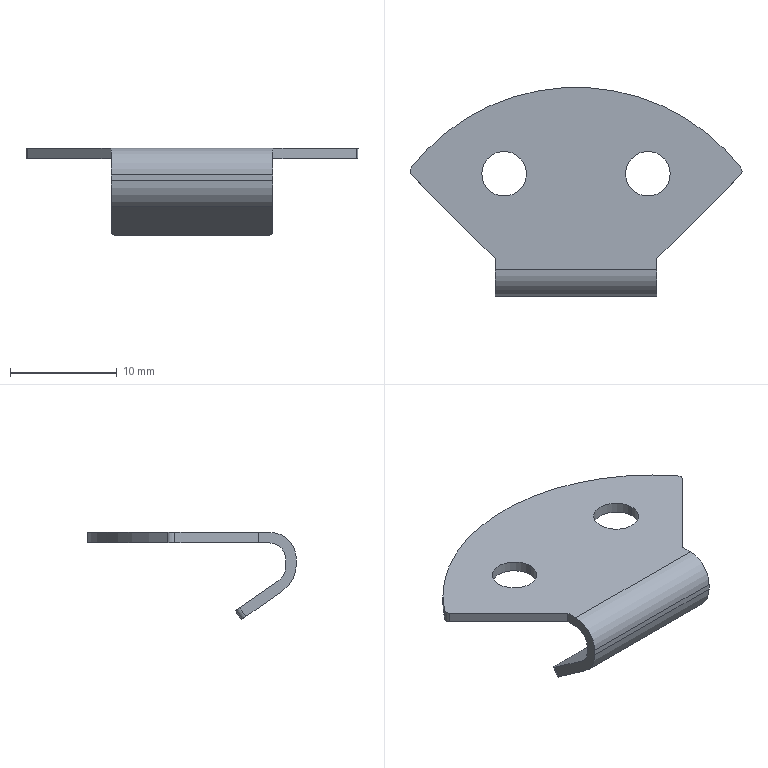Part | SolidWorks | features BaseBody 1 | 1 solid | 24 faces | box 31.176 x 19.62 x 8.2 mm | volume 515.875 mm3 | cylinder 13 | plane 11 | commonest cylinder face diameters 1 x4 4.2 x4 3 x2 5 x1 6 x1 39.24 x1
STEP:
#1=CARTESIAN_POINT('',(8.85,0.,0.));
#2=VERTEX_POINT('',#1);
#3=CARTESIAN_POINT('',(4.65,0.,0.));
#4=VERTEX_POINT('',#3);
#5=CARTESIAN_POINT('',(6.75,0.,0.));
#6=DIRECTION('',(0.,0.,-1.));
#7=DIRECTION('',(-1.,0.,0.));
#8=AXIS2_PLACEMENT_3D('',#5,#6,#7);
#9=CIRCLE('',#8,2.1);
#10=EDGE_CURVE('',#2,#4,#9,.T.);
#11=ORIENTED_EDGE('',*,*,#10,.T.);
#12=CARTESIAN_POINT('',(4.65,0.,1.));
#13=VERTEX_POINT('',#12);
#14=CARTESIAN_POINT('',(4.65,0.,0.));
#15=DIRECTION('',(0.,0.,1.));
#16=VECTOR('',#15,1000.);
#17=LINE('',#14,#16);
#18=EDGE_CURVE('',#4,#13,#17,.T.);
#19=ORIENTED_EDGE('',*,*,#18,.T.);
#20=CARTESIAN_POINT('',(8.85,0.,1.));
#21=VERTEX_POINT('',#20);
#22=CARTESIAN_POINT('',(6.75,0.,1.));
#23=DIRECTION('',(0.,0.,-1.));
#24=DIRECTION('',(1.,0.,0.));
#25=AXIS2_PLACEMENT_3D('',#22,#23,#24);
#26=CIRCLE('',#25,2.1);
#27=EDGE_CURVE('',#21,#13,#26,.T.);
#28=ORIENTED_EDGE('',*,*,#27,.F.);
#29=CARTESIAN_POINT('',(8.85,0.,0.));
#30=DIRECTION('',(0.,0.,1.));
#31=VECTOR('',#30,1000.);
#32=LINE('',#29,#31);
#33=EDGE_CURVE('',#2,#21,#32,.T.);
#34=ORIENTED_EDGE('',*,*,#33,.F.);
#35=EDGE_LOOP('',(#11,#19,#28,#34));
#36=FACE_OUTER_BOUND('',#35,.T.);
#37=CARTESIAN_POINT('',(6.75,0.,0.));
#38=DIRECTION('',(0.,0.,1.));
#39=DIRECTION('',(1.,0.,0.));
#40=AXIS2_PLACEMENT_3D('',#37,#38,#39);
#41=CYLINDRICAL_SURFACE('',#40,2.1);
#42=ADVANCED_FACE('',(#36),#41,.F.);
#43=CARTESIAN_POINT('',(-4.65,0.,0.));
#44=VERTEX_POINT('',#43);
#45=CARTESIAN_POINT('',(-8.85,0.,0.));
#46=VERTEX_POINT('',#45);
#47=CARTESIAN_POINT('',(-6.75,0.,0.));
#48=DIRECTION('',(0.,0.,-1.));
#49=DIRECTION('',(-1.,0.,0.));
#50=AXIS2_PLACEMENT_3D('',#47,#48,#49);
#51=CIRCLE('',#50,2.1);
#52=EDGE_CURVE('',#44,#46,#51,.T.);
#53=ORIENTED_EDGE('',*,*,#52,.T.);
#54=CARTESIAN_POINT('',(-8.85,0.,1.));
#55=VERTEX_POINT('',#54);
#56=CARTESIAN_POINT('',(-8.85,0.,0.));
#57=DIRECTION('',(0.,0.,1.));
#58=VECTOR('',#57,1000.);
#59=LINE('',#56,#58);
#60=EDGE_CURVE('',#46,#55,#59,.T.);
#61=ORIENTED_EDGE('',*,*,#60,.T.);
#62=CARTESIAN_POINT('',(-4.65,0.,1.));
#63=VERTEX_POINT('',#62);
#64=CARTESIAN_POINT('',(-6.75,0.,1.));
#65=DIRECTION('',(0.,0.,-1.));
#66=DIRECTION('',(-1.,0.,0.));
#67=AXIS2_PLACEMENT_3D('',#64,#65,#66);
#68=CIRCLE('',#67,2.1);
#69=EDGE_CURVE('',#63,#55,#68,.T.);
#70=ORIENTED_EDGE('',*,*,#69,.F.);
#71=CARTESIAN_POINT('',(-4.65,0.,0.));
#72=DIRECTION('',(0.,0.,1.));
#73=VECTOR('',#72,1000.);
#74=LINE('',#71,#73);
#75=EDGE_CURVE('',#44,#63,#74,.T.);
#76=ORIENTED_EDGE('',*,*,#75,.F.);
#77=EDGE_LOOP('',(#53,#61,#70,#76));
#78=FACE_OUTER_BOUND('',#77,.T.);
#79=CARTESIAN_POINT('',(-6.75,0.,0.));
#80=DIRECTION('',(0.,0.,1.));
#81=DIRECTION('',(1.,0.,0.));
#82=AXIS2_PLACEMENT_3D('',#79,#80,#81);
#83=CYLINDRICAL_SURFACE('',#82,2.1);
#84=ADVANCED_FACE('',(#78),#83,.F.);
#85=CARTESIAN_POINT('',(-15.441,-0.1087,0.));
#86=VERTEX_POINT('',#85);
#87=CARTESIAN_POINT('',(-7.6,-7.95,0.));
#88=VERTEX_POINT('',#87);
#89=CARTESIAN_POINT('',(-15.441,-0.1087,0.));
#90=DIRECTION('',(0.7071,-0.7071,0.));
#91=VECTOR('',#90,1000.);
#92=LINE('',#89,#91);
#93=EDGE_CURVE('',#86,#88,#92,.T.);
#94=ORIENTED_EDGE('',*,*,#93,.T.);
#95=CARTESIAN_POINT('',(-7.6,-7.95,1.));
#96=VERTEX_POINT('',#95);
#97=CARTESIAN_POINT('',(-7.6,-7.95,0.));
#98=DIRECTION('',(0.,0.,1.));
#99=VECTOR('',#98,1000.);
#100=LINE('',#97,#99);
#101=EDGE_CURVE('',#88,#96,#100,.T.);
#102=ORIENTED_EDGE('',*,*,#101,.T.);
#103=CARTESIAN_POINT('',(-15.441,-0.1087,1.));
#104=VERTEX_POINT('',#103);
#105=CARTESIAN_POINT('',(-15.441,-0.1087,1.));
#106=DIRECTION('',(0.7071,-0.7071,0.));
#107=VECTOR('',#106,1000.);
#108=LINE('',#105,#107);
#109=EDGE_CURVE('',#104,#96,#108,.T.);
#110=ORIENTED_EDGE('',*,*,#109,.F.);
#111=CARTESIAN_POINT('',(-15.441,-0.1087,1.));
#112=DIRECTION('',(0.,0.,-1.));
#113=VECTOR('',#112,1000.);
#114=LINE('',#111,#113);
#115=EDGE_CURVE('',#104,#86,#114,.T.);
#116=ORIENTED_EDGE('',*,*,#115,.T.);
#117=EDGE_LOOP('',(#94,#102,#110,#116));
#118=FACE_OUTER_BOUND('',#117,.T.);
#119=CARTESIAN_POINT('',(-15.75,0.2,0.));
#120=DIRECTION('',(-0.7071,-0.7071,0.));
#121=DIRECTION('',(-0.7071,0.7071,0.));
#122=AXIS2_PLACEMENT_3D('',#119,#120,#121);
#123=PLANE('',#122);
#124=ADVANCED_FACE('',(#118),#123,.T.);
#125=CARTESIAN_POINT('',(-7.6,-9.,1.));
#126=VERTEX_POINT('',#125);
#127=CARTESIAN_POINT('',(7.6,-9.,1.));
#128=VERTEX_POINT('',#127);
#129=CARTESIAN_POINT('',(-7.6,-9.,1.));
#130=DIRECTION('',(1.,0.,0.));
#131=VECTOR('',#130,1000.);
#132=LINE('',#129,#131);
#133=EDGE_CURVE('',#126,#128,#132,.T.);
#134=ORIENTED_EDGE('',*,*,#133,.F.);
#135=CARTESIAN_POINT('',(-7.6,-11.5,-1.5));
#136=VERTEX_POINT('',#135);
#137=CARTESIAN_POINT('',(-7.6,-9.,-1.5));
#138=DIRECTION('',(-1.,0.,0.));
#139=DIRECTION('',(0.,-1.,0.));
#140=AXIS2_PLACEMENT_3D('',#137,#138,#139);
#141=CIRCLE('',#140,2.5);
#142=EDGE_CURVE('',#136,#126,#141,.T.);
#143=ORIENTED_EDGE('',*,*,#142,.F.);
#144=CARTESIAN_POINT('',(7.6,-11.5,-1.5));
#145=VERTEX_POINT('',#144);
#146=CARTESIAN_POINT('',(-7.6,-11.5,-1.5));
#147=DIRECTION('',(1.,0.,0.));
#148=VECTOR('',#147,1000.);
#149=LINE('',#146,#148);
#150=EDGE_CURVE('',#136,#145,#149,.T.);
#151=ORIENTED_EDGE('',*,*,#150,.T.);
#152=CARTESIAN_POINT('',(7.6,-9.,-1.5));
#153=DIRECTION('',(1.,0.,0.));
#154=DIRECTION('',(0.,0.,1.));
#155=AXIS2_PLACEMENT_3D('',#152,#153,#154);
#156=CIRCLE('',#155,2.5);
#157=EDGE_CURVE('',#128,#145,#156,.T.);
#158=ORIENTED_EDGE('',*,*,#157,.F.);
#159=EDGE_LOOP('',(#134,#143,#151,#158));
#160=FACE_OUTER_BOUND('',#159,.T.);
#161=CARTESIAN_POINT('',(-56.813,-9.,-1.5));
#162=DIRECTION('',(1.,0.,0.));
#163=DIRECTION('',(0.,0.,1.));
#164=AXIS2_PLACEMENT_3D('',#161,#162,#163);
#165=CYLINDRICAL_SURFACE('',#164,2.5);
#166=ADVANCED_FACE('',(#160),#165,.T.);
#167=CARTESIAN_POINT('',(7.6,-11.5,-2.037));
#168=VERTEX_POINT('',#167);
#169=CARTESIAN_POINT('',(7.6,-11.5,-1.5));
#170=DIRECTION('',(0.,0.,-1.));
#171=VECTOR('',#170,1000.);
#172=LINE('',#169,#171);
#173=EDGE_CURVE('',#145,#168,#172,.T.);
#174=ORIENTED_EDGE('',*,*,#173,.F.);
#175=ORIENTED_EDGE('',*,*,#150,.F.);
#176=CARTESIAN_POINT('',(-7.6,-11.5,-2.037));
#177=VERTEX_POINT('',#176);
#178=CARTESIAN_POINT('',(-7.6,-11.5,-2.037));
#179=DIRECTION('',(0.,0.,1.));
#180=VECTOR('',#179,1000.);
#181=LINE('',#178,#180);
#182=EDGE_CURVE('',#177,#136,#181,.T.);
#183=ORIENTED_EDGE('',*,*,#182,.F.);
#184=CARTESIAN_POINT('',(7.6,-11.5,-2.037));
#185=DIRECTION('',(-1.,0.,0.));
#186=VECTOR('',#185,1000.);
#187=LINE('',#184,#186);
#188=EDGE_CURVE('',#168,#177,#187,.T.);
#189=ORIENTED_EDGE('',*,*,#188,.F.);
#190=EDGE_LOOP('',(#174,#175,#183,#189));
#191=FACE_OUTER_BOUND('',#190,.T.);
#192=CARTESIAN_POINT('',(-7.6,-11.5,0.));
#193=DIRECTION('',(0.,-1.,0.));
#194=DIRECTION('',(0.,0.,-1.));
#195=AXIS2_PLACEMENT_3D('',#192,#193,#194);
#196=PLANE('',#195);
#197=ADVANCED_FACE('',(#191),#196,.T.);
#198=CARTESIAN_POINT('',(7.6,-10.219,-4.496));
#199=VERTEX_POINT('',#198);
#200=CARTESIAN_POINT('',(-7.6,-10.219,-4.496));
#201=VERTEX_POINT('',#200);
#202=CARTESIAN_POINT('',(7.6,-10.219,-4.496));
#203=DIRECTION('',(-1.,0.,0.));
#204=VECTOR('',#203,1000.);
#205=LINE('',#202,#204);
#206=EDGE_CURVE('',#199,#201,#205,.T.);
#207=ORIENTED_EDGE('',*,*,#206,.F.);
#208=CARTESIAN_POINT('',(7.6,-8.5,-2.037));
#209=DIRECTION('',(1.,0.,0.));
#210=DIRECTION('',(0.,-1.,0.));
#211=AXIS2_PLACEMENT_3D('',#208,#209,#210);
#212=CIRCLE('',#211,3.);
#213=EDGE_CURVE('',#168,#199,#212,.T.);
#214=ORIENTED_EDGE('',*,*,#213,.F.);
#215=ORIENTED_EDGE('',*,*,#188,.T.);
#216=CARTESIAN_POINT('',(-7.6,-8.5,-2.037));
#217=DIRECTION('',(-1.,0.,0.));
#218=DIRECTION('',(0.,-0.5732,-0.8194));
#219=AXIS2_PLACEMENT_3D('',#216,#217,#218);
#220=CIRCLE('',#219,3.);
#221=EDGE_CURVE('',#201,#177,#220,.T.);
#222=ORIENTED_EDGE('',*,*,#221,.F.);
#223=EDGE_LOOP('',(#207,#214,#215,#222));
#224=FACE_OUTER_BOUND('',#223,.T.);
#225=CARTESIAN_POINT('',(56.813,-8.5,-2.037));
#226=DIRECTION('',(-1.,0.,0.));
#227=DIRECTION('',(0.,-0.5732,-0.8194));
#228=AXIS2_PLACEMENT_3D('',#225,#226,#227);
#229=CYLINDRICAL_SURFACE('',#228,3.);
#230=ADVANCED_FACE('',(#224),#229,.T.);
#231=CARTESIAN_POINT('',(-7.1,-6.353,-7.2));
#232=VERTEX_POINT('',#231);
#233=CARTESIAN_POINT('',(7.1,-6.353,-7.2));
#234=VERTEX_POINT('',#233);
#235=CARTESIAN_POINT('',(-7.1,-6.353,-7.2));
#236=DIRECTION('',(1.,0.,0.));
#237=VECTOR('',#236,1000.);
#238=LINE('',#235,#237);
#239=EDGE_CURVE('',#232,#234,#238,.T.);
#240=ORIENTED_EDGE('',*,*,#239,.F.);
#241=CARTESIAN_POINT('',(-7.1,-5.78,-6.381));
#242=VERTEX_POINT('',#241);
#243=CARTESIAN_POINT('',(-7.1,-5.78,-6.381));
#244=DIRECTION('',(0.,-0.5732,-0.8194));
#245=VECTOR('',#244,1000.);
#246=LINE('',#243,#245);
#247=EDGE_CURVE('',#242,#232,#246,.T.);
#248=ORIENTED_EDGE('',*,*,#247,.F.);
#249=CARTESIAN_POINT('',(7.1,-5.78,-6.381));
#250=VERTEX_POINT('',#249);
#251=CARTESIAN_POINT('',(-7.1,-5.78,-6.381));
#252=DIRECTION('',(1.,0.,0.));
#253=VECTOR('',#252,1000.);
#254=LINE('',#251,#253);
#255=EDGE_CURVE('',#242,#250,#254,.T.);
#256=ORIENTED_EDGE('',*,*,#255,.T.);
#257=CARTESIAN_POINT('',(7.1,-6.353,-7.2));
#258=DIRECTION('',(0.,0.5732,0.8194));
#259=VECTOR('',#258,1000.);
#260=LINE('',#257,#259);
#261=EDGE_CURVE('',#234,#250,#260,.T.);
#262=ORIENTED_EDGE('',*,*,#261,.F.);
#263=EDGE_LOOP('',(#240,#248,#256,#262));
#264=FACE_OUTER_BOUND('',#263,.T.);
#265=CARTESIAN_POINT('',(-7.6,-6.353,-7.2));
#266=DIRECTION('',(0.,0.8194,-0.5732));
#267=DIRECTION('',(-1.,0.,0.));
#268=AXIS2_PLACEMENT_3D('',#265,#266,#267);
#269=PLANE('',#268);
#270=ADVANCED_FACE('',(#264),#269,.T.);
#271=CARTESIAN_POINT('',(7.6,-6.763,-6.913));
#272=VERTEX_POINT('',#271);
#273=CARTESIAN_POINT('',(7.6,-10.219,-4.496));
#274=DIRECTION('',(0.,0.8194,-0.5732));
#275=VECTOR('',#274,1000.);
#276=LINE('',#273,#275);
#277=EDGE_CURVE('',#199,#272,#276,.T.);
#278=ORIENTED_EDGE('',*,*,#277,.F.);
#279=ORIENTED_EDGE('',*,*,#206,.T.);
#280=CARTESIAN_POINT('',(-7.6,-6.763,-6.913));
#281=VERTEX_POINT('',#280);
#282=CARTESIAN_POINT('',(-7.6,-10.219,-4.496));
#283=DIRECTION('',(0.,0.8194,-0.5732));
#284=VECTOR('',#283,1000.);
#285=LINE('',#282,#284);
#286=EDGE_CURVE('',#201,#281,#285,.T.);
#287=ORIENTED_EDGE('',*,*,#286,.T.);
#288=CARTESIAN_POINT('',(-7.1,-6.763,-6.913));
#289=DIRECTION('',(0.,-0.5732,-0.8194));
#290=DIRECTION('',(-1.,0.,0.));
#291=AXIS2_PLACEMENT_3D('',#288,#289,#290);
#292=CIRCLE('',#291,0.5);
#293=EDGE_CURVE('',#281,#232,#292,.T.);
#294=ORIENTED_EDGE('',*,*,#293,.T.);
#295=ORIENTED_EDGE('',*,*,#239,.T.);
#296=CARTESIAN_POINT('',(7.1,-6.763,-6.913));
#297=DIRECTION('',(0.,-0.5732,-0.8194));
#298=DIRECTION('',(0.,0.8194,-0.5732));
#299=AXIS2_PLACEMENT_3D('',#296,#297,#298);
#300=CIRCLE('',#299,0.5);
#301=EDGE_CURVE('',#234,#272,#300,.T.);
#302=ORIENTED_EDGE('',*,*,#301,.T.);
#303=EDGE_LOOP('',(#278,#279,#287,#294,#295,#302));
#304=FACE_OUTER_BOUND('',#303,.T.);
#305=CARTESIAN_POINT('',(-7.6,-11.5,-3.6));
#306=DIRECTION('',(0.,-0.5732,-0.8194));
#307=DIRECTION('',(0.,-0.8194,0.5732));
#308=AXIS2_PLACEMENT_3D('',#305,#306,#307);
#309=PLANE('',#308);
#310=ADVANCED_FACE('',(#304),#309,.T.);
#311=CARTESIAN_POINT('',(-7.6,-6.19,-6.094));
#312=VERTEX_POINT('',#311);
#313=CARTESIAN_POINT('',(-7.6,-6.19,-6.094));
#314=DIRECTION('',(0.,-0.5732,-0.8194));
#315=VECTOR('',#314,1000.);
#316=LINE('',#313,#315);
#317=EDGE_CURVE('',#312,#281,#316,.T.);
#318=ORIENTED_EDGE('',*,*,#317,.F.);
#319=CARTESIAN_POINT('',(-7.1,-6.19,-6.094));
#320=DIRECTION('',(0.,0.5732,0.8194));
#321=DIRECTION('',(0.,0.8194,-0.5732));
#322=AXIS2_PLACEMENT_3D('',#319,#320,#321);
#323=CIRCLE('',#322,0.5);
#324=EDGE_CURVE('',#242,#312,#323,.T.);
#325=ORIENTED_EDGE('',*,*,#324,.F.);
#326=ORIENTED_EDGE('',*,*,#247,.T.);
#327=ORIENTED_EDGE('',*,*,#293,.F.);
#328=EDGE_LOOP('',(#318,#325,#326,#327));
#329=FACE_OUTER_BOUND('',#328,.T.);
#330=CARTESIAN_POINT('',(-7.1,6.249,11.69));
#331=DIRECTION('',(0.,-0.5732,-0.8194));
#332=DIRECTION('',(-1.,0.,0.));
#333=AXIS2_PLACEMENT_3D('',#330,#331,#332);
#334=CYLINDRICAL_SURFACE('',#333,0.5);
#335=ADVANCED_FACE('',(#329),#334,.T.);
#336=ORIENTED_EDGE('',*,*,#286,.F.);
#337=ORIENTED_EDGE('',*,*,#221,.T.);
#338=ORIENTED_EDGE('',*,*,#182,.T.);
#339=ORIENTED_EDGE('',*,*,#142,.T.);
#340=CARTESIAN_POINT('',(-7.6,-7.95,1.));
#341=DIRECTION('',(0.,-1.,0.));
#342=VECTOR('',#341,1000.);
#343=LINE('',#340,#342);
#344=EDGE_CURVE('',#96,#126,#343,.T.);
#345=ORIENTED_EDGE('',*,*,#344,.F.);
#346=ORIENTED_EDGE('',*,*,#101,.F.);
#347=CARTESIAN_POINT('',(-7.6,-9.,0.));
#348=VERTEX_POINT('',#347);
#349=CARTESIAN_POINT('',(-7.6,-7.95,0.));
#350=DIRECTION('',(0.,-1.,0.));
#351=VECTOR('',#350,1000.);
#352=LINE('',#349,#351);
#353=EDGE_CURVE('',#88,#348,#352,.T.);
#354=ORIENTED_EDGE('',*,*,#353,.T.);
#355=CARTESIAN_POINT('',(-7.6,-10.5,-1.5));
#356=VERTEX_POINT('',#355);
#357=CARTESIAN_POINT('',(-7.6,-9.,-1.5));
#358=DIRECTION('',(1.,0.,0.));
#359=DIRECTION('',(0.,0.,1.));
#360=AXIS2_PLACEMENT_3D('',#357,#358,#359);
#361=CIRCLE('',#360,1.5);
#362=EDGE_CURVE('',#348,#356,#361,.T.);
#363=ORIENTED_EDGE('',*,*,#362,.T.);
#364=CARTESIAN_POINT('',(-7.6,-10.5,-2.298));
#365=VERTEX_POINT('',#364);
#366=CARTESIAN_POINT('',(-7.6,-10.5,-2.298));
#367=DIRECTION('',(0.,0.,1.));
#368=VECTOR('',#367,1000.);
#369=LINE('',#366,#368);
#370=EDGE_CURVE('',#365,#356,#369,.T.);
#371=ORIENTED_EDGE('',*,*,#370,.F.);
#372=CARTESIAN_POINT('',(-7.6,-9.86,-3.527));
#373=VERTEX_POINT('',#372);
#374=CARTESIAN_POINT('',(-7.6,-9.,-2.298));
#375=DIRECTION('',(1.,0.,0.));
#376=DIRECTION('',(0.,-1.,0.));
#377=AXIS2_PLACEMENT_3D('',#374,#375,#376);
#378=CIRCLE('',#377,1.5);
#379=EDGE_CURVE('',#365,#373,#378,.T.);
#380=ORIENTED_EDGE('',*,*,#379,.T.);
#381=CARTESIAN_POINT('',(-7.6,-6.19,-6.094));
#382=DIRECTION('',(0.,-0.8194,0.5732));
#383=VECTOR('',#382,1000.);
#384=LINE('',#381,#383);
#385=EDGE_CURVE('',#312,#373,#384,.T.);
#386=ORIENTED_EDGE('',*,*,#385,.F.);
#387=ORIENTED_EDGE('',*,*,#317,.T.);
#388=EDGE_LOOP('',(#336,#337,#338,#339,#345,#346,#354,#363,#371,#380,#386,#387));
#389=FACE_OUTER_BOUND('',#388,.T.);
#390=CARTESIAN_POINT('',(-7.6,-7.95,0.));
#391=DIRECTION('',(-1.,0.,0.));
#392=DIRECTION('',(0.,0.,1.));
#393=AXIS2_PLACEMENT_3D('',#390,#391,#392);
#394=PLANE('',#393);
#395=ADVANCED_FACE('',(#389),#394,.T.);
#396=CARTESIAN_POINT('',(7.6,-10.5,-1.5));
#397=VERTEX_POINT('',#396);
#398=CARTESIAN_POINT('',(7.6,-9.,0.));
#399=VERTEX_POINT('',#398);
#400=CARTESIAN_POINT('',(7.6,-9.,-1.5));
#401=DIRECTION('',(-1.,0.,0.));
#402=DIRECTION('',(0.,-1.,0.));
#403=AXIS2_PLACEMENT_3D('',#400,#401,#402);
#404=CIRCLE('',#403,1.5);
#405=EDGE_CURVE('',#397,#399,#404,.T.);
#406=ORIENTED_EDGE('',*,*,#405,.F.);
#407=CARTESIAN_POINT('',(-7.6,-10.5,-1.5));
#408=DIRECTION('',(1.,0.,0.));
#409=VECTOR('',#408,1000.);
#410=LINE('',#407,#409);
#411=EDGE_CURVE('',#356,#397,#410,.T.);
#412=ORIENTED_EDGE('',*,*,#411,.F.);
#413=ORIENTED_EDGE('',*,*,#362,.F.);
#414=CARTESIAN_POINT('',(-7.6,-9.,0.));
#415=DIRECTION('',(1.,0.,0.));
#416=VECTOR('',#415,1000.);
#417=LINE('',#414,#416);
#418=EDGE_CURVE('',#348,#399,#417,.T.);
#419=ORIENTED_EDGE('',*,*,#418,.T.);
#420=EDGE_LOOP('',(#406,#412,#413,#419));
#421=FACE_OUTER_BOUND('',#420,.T.);
#422=CARTESIAN_POINT('',(-56.813,-9.,-1.5));
#423=DIRECTION('',(1.,0.,0.));
#424=DIRECTION('',(0.,0.,1.));
#425=AXIS2_PLACEMENT_3D('',#422,#423,#424);
#426=CYLINDRICAL_SURFACE('',#425,1.5);
#427=ADVANCED_FACE('',(#421),#426,.F.);
#428=CARTESIAN_POINT('',(7.6,-10.5,-2.298));
#429=VERTEX_POINT('',#428);
#430=CARTESIAN_POINT('',(7.6,-10.5,-2.298));
#431=DIRECTION('',(0.,0.,1.));
#432=VECTOR('',#431,1000.);
#433=LINE('',#430,#432);
#434=EDGE_CURVE('',#429,#397,#433,.T.);
#435=ORIENTED_EDGE('',*,*,#434,.F.);
#436=CARTESIAN_POINT('',(-7.6,-10.5,-2.298));
#437=DIRECTION('',(1.,0.,0.));
#438=VECTOR('',#437,1000.);
#439=LINE('',#436,#438);
#440=EDGE_CURVE('',#365,#429,#439,.T.);
#441=ORIENTED_EDGE('',*,*,#440,.F.);
#442=ORIENTED_EDGE('',*,*,#370,.T.);
#443=ORIENTED_EDGE('',*,*,#411,.T.);
#444=EDGE_LOOP('',(#435,#441,#442,#443));
#445=FACE_OUTER_BOUND('',#444,.T.);
#446=CARTESIAN_POINT('',(-7.6,-10.5,-3.079));
#447=DIRECTION('',(0.,1.,0.));
#448=DIRECTION('',(1.,0.,0.));
#449=AXIS2_PLACEMENT_3D('',#446,#447,#448);
#450=PLANE('',#449);
#451=ADVANCED_FACE('',(#445),#450,.T.);
#452=CARTESIAN_POINT('',(7.6,-9.86,-3.527));
#453=VERTEX_POINT('',#452);
#454=CARTESIAN_POINT('',(7.6,-9.,-2.298));
#455=DIRECTION('',(-1.,0.,0.));
#456=DIRECTION('',(0.,-0.5732,-0.8194));
#457=AXIS2_PLACEMENT_3D('',#454,#455,#456);
#458=CIRCLE('',#457,1.5);
#459=EDGE_CURVE('',#453,#429,#458,.T.);
#460=ORIENTED_EDGE('',*,*,#459,.F.);
#461=CARTESIAN_POINT('',(-7.6,-9.86,-3.527));
#462=DIRECTION('',(1.,0.,0.));
#463=VECTOR('',#462,1000.);
#464=LINE('',#461,#463);
#465=EDGE_CURVE('',#373,#453,#464,.T.);
#466=ORIENTED_EDGE('',*,*,#465,.F.);
#467=ORIENTED_EDGE('',*,*,#379,.F.);
#468=ORIENTED_EDGE('',*,*,#440,.T.);
#469=EDGE_LOOP('',(#460,#466,#467,#468));
#470=FACE_OUTER_BOUND('',#469,.T.);
#471=CARTESIAN_POINT('',(-56.813,-9.,-2.298));
#472=DIRECTION('',(1.,0.,0.));
#473=DIRECTION('',(0.,-1.,0.));
#474=AXIS2_PLACEMENT_3D('',#471,#472,#473);
#475=CYLINDRICAL_SURFACE('',#474,1.5);
#476=ADVANCED_FACE('',(#470),#475,.F.);
#477=ORIENTED_EDGE('',*,*,#255,.F.);
#478=ORIENTED_EDGE('',*,*,#324,.T.);
#479=ORIENTED_EDGE('',*,*,#385,.T.);
#480=ORIENTED_EDGE('',*,*,#465,.T.);
#481=CARTESIAN_POINT('',(7.6,-6.19,-6.094));
#482=VERTEX_POINT('',#481);
#483=CARTESIAN_POINT('',(7.6,-6.19,-6.094));
#484=DIRECTION('',(0.,-0.8194,0.5732));
#485=VECTOR('',#484,1000.);
#486=LINE('',#483,#485);
#487=EDGE_CURVE('',#482,#453,#486,.T.);
#488=ORIENTED_EDGE('',*,*,#487,.F.);
#489=CARTESIAN_POINT('',(7.1,-6.19,-6.094));
#490=DIRECTION('',(0.,0.5732,0.8194));
#491=DIRECTION('',(1.,0.,0.));
#492=AXIS2_PLACEMENT_3D('',#489,#490,#491);
#493=CIRCLE('',#492,0.5);
#494=EDGE_CURVE('',#482,#250,#493,.T.);
#495=ORIENTED_EDGE('',*,*,#494,.T.);
#496=EDGE_LOOP('',(#477,#478,#479,#480,#488,#495));
#497=FACE_OUTER_BOUND('',#496,.T.);
#498=CARTESIAN_POINT('',(-7.6,-5.78,-6.381));
#499=DIRECTION('',(0.,0.5732,0.8194));
#500=DIRECTION('',(1.,0.,0.));
#501=AXIS2_PLACEMENT_3D('',#498,#499,#500);
#502=PLANE('',#501);
#503=ADVANCED_FACE('',(#497),#502,.T.);
#504=CARTESIAN_POINT('',(7.6,-6.763,-6.913));
#505=DIRECTION('',(0.,0.5732,0.8194));
#506=VECTOR('',#505,1000.);
#507=LINE('',#504,#506);
#508=EDGE_CURVE('',#272,#482,#507,.T.);
#509=ORIENTED_EDGE('',*,*,#508,.F.);
#510=ORIENTED_EDGE('',*,*,#301,.F.);
#511=ORIENTED_EDGE('',*,*,#261,.T.);
#512=ORIENTED_EDGE('',*,*,#494,.F.);
#513=EDGE_LOOP('',(#509,#510,#511,#512));
#514=FACE_OUTER_BOUND('',#513,.T.);
#515=CARTESIAN_POINT('',(7.1,-14.44,-17.89));
#516=DIRECTION('',(0.,0.5732,0.8194));
#517=DIRECTION('',(1.,0.,0.));
#518=AXIS2_PLACEMENT_3D('',#515,#516,#517);
#519=CYLINDRICAL_SURFACE('',#518,0.5);
#520=ADVANCED_FACE('',(#514),#519,.T.);
#521=ORIENTED_EDGE('',*,*,#487,.T.);
#522=ORIENTED_EDGE('',*,*,#459,.T.);
#523=ORIENTED_EDGE('',*,*,#434,.T.);
#524=ORIENTED_EDGE('',*,*,#405,.T.);
#525=CARTESIAN_POINT('',(7.6,-7.95,0.));
#526=VERTEX_POINT('',#525);
#527=CARTESIAN_POINT('',(7.6,-9.,0.));
#528=DIRECTION('',(0.,1.,0.));
#529=VECTOR('',#528,1000.);
#530=LINE('',#527,#529);
#531=EDGE_CURVE('',#399,#526,#530,.T.);
#532=ORIENTED_EDGE('',*,*,#531,.T.);
#533=CARTESIAN_POINT('',(7.6,-7.95,1.));
#534=VERTEX_POINT('',#533);
#535=CARTESIAN_POINT('',(7.6,-7.95,0.));
#536=DIRECTION('',(0.,0.,1.));
#537=VECTOR('',#536,1000.);
#538=LINE('',#535,#537);
#539=EDGE_CURVE('',#526,#534,#538,.T.);
#540=ORIENTED_EDGE('',*,*,#539,.T.);
#541=CARTESIAN_POINT('',(7.6,-9.,1.));
#542=DIRECTION('',(0.,1.,0.));
#543=VECTOR('',#542,1000.);
#544=LINE('',#541,#543);
#545=EDGE_CURVE('',#128,#534,#544,.T.);
#546=ORIENTED_EDGE('',*,*,#545,.F.);
#547=ORIENTED_EDGE('',*,*,#157,.T.);
#548=ORIENTED_EDGE('',*,*,#173,.T.);
#549=ORIENTED_EDGE('',*,*,#213,.T.);
#550=ORIENTED_EDGE('',*,*,#277,.T.);
#551=ORIENTED_EDGE('',*,*,#508,.T.);
#552=EDGE_LOOP('',(#521,#522,#523,#524,#532,#540,#546,#547,#548,#549,#550,#551));
#553=FACE_OUTER_BOUND('',#552,.T.);
#554=CARTESIAN_POINT('',(7.6,-11.5,0.));
#555=DIRECTION('',(1.,0.,0.));
#556=DIRECTION('',(0.,1.,0.));
#557=AXIS2_PLACEMENT_3D('',#554,#555,#556);
#558=PLANE('',#557);
#559=ADVANCED_FACE('',(#553),#558,.T.);
#560=CARTESIAN_POINT('',(15.441,-0.1087,1.));
#561=VERTEX_POINT('',#560);
#562=CARTESIAN_POINT('',(7.6,-7.95,1.));
#563=DIRECTION('',(0.7071,0.7071,0.));
#564=VECTOR('',#563,1000.);
#565=LINE('',#562,#564);
#566=EDGE_CURVE('',#534,#561,#565,.T.);
#567=ORIENTED_EDGE('',*,*,#566,.F.);
#568=ORIENTED_EDGE('',*,*,#539,.F.);
#569=CARTESIAN_POINT('',(15.441,-0.1087,0.));
#570=VERTEX_POINT('',#569);
#571=CARTESIAN_POINT('',(7.6,-7.95,0.));
#572=DIRECTION('',(0.7071,0.7071,0.));
#573=VECTOR('',#572,1000.);
#574=LINE('',#571,#573);
#575=EDGE_CURVE('',#526,#570,#574,.T.);
#576=ORIENTED_EDGE('',*,*,#575,.T.);
#577=CARTESIAN_POINT('',(15.441,-0.1087,1.));
#578=DIRECTION('',(0.,0.,-1.));
#579=VECTOR('',#578,1000.);
#580=LINE('',#577,#579);
#581=EDGE_CURVE('',#561,#570,#580,.T.);
#582=ORIENTED_EDGE('',*,*,#581,.F.);
#583=EDGE_LOOP('',(#567,#568,#576,#582));
#584=FACE_OUTER_BOUND('',#583,.T.);
#585=CARTESIAN_POINT('',(7.6,-7.95,0.));
#586=DIRECTION('',(0.7071,-0.7071,0.));
#587=DIRECTION('',(0.,0.,-1.));
#588=AXIS2_PLACEMENT_3D('',#585,#586,#587);
#589=PLANE('',#588);
#590=ADVANCED_FACE('',(#584),#589,.T.);
#591=CARTESIAN_POINT('',(15.482,0.552,1.));
#592=VERTEX_POINT('',#591);
#593=CARTESIAN_POINT('',(15.482,0.552,0.));
#594=VERTEX_POINT('',#593);
#595=CARTESIAN_POINT('',(15.482,0.552,1.));
#596=DIRECTION('',(0.,0.,-1.));
#597=VECTOR('',#596,1000.);
#598=LINE('',#595,#597);
#599=EDGE_CURVE('',#592,#594,#598,.T.);
#600=ORIENTED_EDGE('',*,*,#599,.F.);
#601=CARTESIAN_POINT('',(15.088,0.2449,1.));
#602=DIRECTION('',(0.,0.,1.));
#603=DIRECTION('',(0.7071,-0.7071,0.));
#604=AXIS2_PLACEMENT_3D('',#601,#602,#603);
#605=CIRCLE('',#604,0.5);
#606=EDGE_CURVE('',#561,#592,#605,.T.);
#607=ORIENTED_EDGE('',*,*,#606,.F.);
#608=ORIENTED_EDGE('',*,*,#581,.T.);
#609=CARTESIAN_POINT('',(15.088,0.2449,0.));
#610=DIRECTION('',(0.,0.,-1.));
#611=DIRECTION('',(0.7891,0.6143,0.));
#612=AXIS2_PLACEMENT_3D('',#609,#610,#611);
#613=CIRCLE('',#612,0.5);
#614=EDGE_CURVE('',#594,#570,#613,.T.);
#615=ORIENTED_EDGE('',*,*,#614,.F.);
#616=EDGE_LOOP('',(#600,#607,#608,#615));
#617=FACE_OUTER_BOUND('',#616,.T.);
#618=CARTESIAN_POINT('',(15.088,0.2449,11.69));
#619=DIRECTION('',(0.,0.,-1.));
#620=DIRECTION('',(0.7891,0.6143,0.));
#621=AXIS2_PLACEMENT_3D('',#618,#619,#620);
#622=CYLINDRICAL_SURFACE('',#621,0.5);
#623=ADVANCED_FACE('',(#617),#622,.T.);
#624=CARTESIAN_POINT('',(-15.482,0.552,1.));
#625=VERTEX_POINT('',#624);
#626=CARTESIAN_POINT('',(0.,-11.5,1.));
#627=DIRECTION('',(0.,0.,1.));
#628=DIRECTION('',(0.7891,0.6143,0.));
#629=AXIS2_PLACEMENT_3D('',#626,#627,#628);
#630=CIRCLE('',#629,19.62);
#631=EDGE_CURVE('',#592,#625,#630,.T.);
#632=ORIENTED_EDGE('',*,*,#631,.F.);
#633=ORIENTED_EDGE('',*,*,#599,.T.);
#634=CARTESIAN_POINT('',(-15.482,0.552,0.));
#635=VERTEX_POINT('',#634);
#636=CARTESIAN_POINT('',(0.,-11.5,0.));
#637=DIRECTION('',(0.,0.,1.));
#638=DIRECTION('',(0.7891,0.6143,0.));
#639=AXIS2_PLACEMENT_3D('',#636,#637,#638);
#640=CIRCLE('',#639,19.62);
#641=EDGE_CURVE('',#594,#635,#640,.T.);
#642=ORIENTED_EDGE('',*,*,#641,.T.);
#643=CARTESIAN_POINT('',(-15.482,0.552,1.));
#644=DIRECTION('',(0.,0.,-1.));
#645=VECTOR('',#644,1000.);
#646=LINE('',#643,#645);
#647=EDGE_CURVE('',#625,#635,#646,.T.);
#648=ORIENTED_EDGE('',*,*,#647,.F.);
#649=EDGE_LOOP('',(#632,#633,#642,#648));
#650=FACE_OUTER_BOUND('',#649,.T.);
#651=CARTESIAN_POINT('',(0.,-11.5,0.));
#652=DIRECTION('',(0.,0.,1.));
#653=DIRECTION('',(1.,0.,0.));
#654=AXIS2_PLACEMENT_3D('',#651,#652,#653);
#655=CYLINDRICAL_SURFACE('',#654,19.62);
#656=ADVANCED_FACE('',(#650),#655,.T.);
#657=ORIENTED_EDGE('',*,*,#115,.F.);
#658=CARTESIAN_POINT('',(-15.088,0.2449,1.));
#659=DIRECTION('',(0.,0.,1.));
#660=DIRECTION('',(-0.7891,0.6143,0.));
#661=AXIS2_PLACEMENT_3D('',#658,#659,#660);
#662=CIRCLE('',#661,0.5);
#663=EDGE_CURVE('',#625,#104,#662,.T.);
#664=ORIENTED_EDGE('',*,*,#663,.F.);
#665=ORIENTED_EDGE('',*,*,#647,.T.);
#666=CARTESIAN_POINT('',(-15.088,0.2449,0.));
#667=DIRECTION('',(0.,0.,-1.));
#668=DIRECTION('',(-0.7071,-0.7071,0.));
#669=AXIS2_PLACEMENT_3D('',#666,#667,#668);
#670=CIRCLE('',#669,0.5);
#671=EDGE_CURVE('',#86,#635,#670,.T.);
#672=ORIENTED_EDGE('',*,*,#671,.F.);
#673=EDGE_LOOP('',(#657,#664,#665,#672));
#674=FACE_OUTER_BOUND('',#673,.T.);
#675=CARTESIAN_POINT('',(-15.088,0.2449,11.69));
#676=DIRECTION('',(0.,0.,-1.));
#677=DIRECTION('',(-0.7071,-0.7071,0.));
#678=AXIS2_PLACEMENT_3D('',#675,#676,#677);
#679=CYLINDRICAL_SURFACE('',#678,0.5);
#680=ADVANCED_FACE('',(#674),#679,.T.);
#681=ORIENTED_EDGE('',*,*,#60,.F.);
#682=CARTESIAN_POINT('',(-6.75,0.,0.));
#683=DIRECTION('',(0.,0.,-1.));
#684=DIRECTION('',(-1.,0.,0.));
#685=AXIS2_PLACEMENT_3D('',#682,#683,#684);
#686=CIRCLE('',#685,2.1);
#687=EDGE_CURVE('',#46,#44,#686,.T.);
#688=ORIENTED_EDGE('',*,*,#687,.T.);
#689=ORIENTED_EDGE('',*,*,#75,.T.);
#690=CARTESIAN_POINT('',(-6.75,0.,1.));
#691=DIRECTION('',(0.,0.,-1.));
#692=DIRECTION('',(-1.,0.,0.));
#693=AXIS2_PLACEMENT_3D('',#690,#691,#692);
#694=CIRCLE('',#693,2.1);
#695=EDGE_CURVE('',#55,#63,#694,.T.);
#696=ORIENTED_EDGE('',*,*,#695,.F.);
#697=EDGE_LOOP('',(#681,#688,#689,#696));
#698=FACE_OUTER_BOUND('',#697,.T.);
#699=CARTESIAN_POINT('',(-6.75,0.,0.));
#700=DIRECTION('',(0.,0.,1.));
#701=DIRECTION('',(1.,0.,0.));
#702=AXIS2_PLACEMENT_3D('',#699,#700,#701);
#703=CYLINDRICAL_SURFACE('',#702,2.1);
#704=ADVANCED_FACE('',(#698),#703,.F.);
#705=ORIENTED_EDGE('',*,*,#69,.T.);
#706=ORIENTED_EDGE('',*,*,#695,.T.);
#707=EDGE_LOOP('',(#705,#706));
#708=FACE_BOUND('',#707,.T.);
#709=ORIENTED_EDGE('',*,*,#27,.T.);
#710=CARTESIAN_POINT('',(6.75,0.,1.));
#711=DIRECTION('',(0.,0.,-1.));
#712=DIRECTION('',(1.,0.,0.));
#713=AXIS2_PLACEMENT_3D('',#710,#711,#712);
#714=CIRCLE('',#713,2.1);
#715=EDGE_CURVE('',#13,#21,#714,.T.);
#716=ORIENTED_EDGE('',*,*,#715,.T.);
#717=EDGE_LOOP('',(#709,#716));
#718=FACE_BOUND('',#717,.T.);
#719=ORIENTED_EDGE('',*,*,#109,.T.);
#720=ORIENTED_EDGE('',*,*,#344,.T.);
#721=ORIENTED_EDGE('',*,*,#133,.T.);
#722=ORIENTED_EDGE('',*,*,#545,.T.);
#723=ORIENTED_EDGE('',*,*,#566,.T.);
#724=ORIENTED_EDGE('',*,*,#606,.T.);
#725=ORIENTED_EDGE('',*,*,#631,.T.);
#726=ORIENTED_EDGE('',*,*,#663,.T.);
#727=EDGE_LOOP('',(#719,#720,#721,#722,#723,#724,#725,#726));
#728=FACE_OUTER_BOUND('',#727,.T.);
#729=CARTESIAN_POINT('',(0.,0.,1.));
#730=DIRECTION('',(0.,0.,1.));
#731=DIRECTION('',(1.,0.,0.));
#732=AXIS2_PLACEMENT_3D('',#729,#730,#731);
#733=PLANE('',#732);
#734=ADVANCED_FACE('',(#708,#718,#728),#733,.T.);
#735=ORIENTED_EDGE('',*,*,#18,.F.);
#736=CARTESIAN_POINT('',(6.75,0.,0.));
#737=DIRECTION('',(0.,0.,-1.));
#738=DIRECTION('',(-1.,0.,0.));
#739=AXIS2_PLACEMENT_3D('',#736,#737,#738);
#740=CIRCLE('',#739,2.1);
#741=EDGE_CURVE('',#4,#2,#740,.T.);
#742=ORIENTED_EDGE('',*,*,#741,.T.);
#743=ORIENTED_EDGE('',*,*,#33,.T.);
#744=ORIENTED_EDGE('',*,*,#715,.F.);
#745=EDGE_LOOP('',(#735,#742,#743,#744));
#746=FACE_OUTER_BOUND('',#745,.T.);
#747=CARTESIAN_POINT('',(6.75,0.,0.));
#748=DIRECTION('',(0.,0.,1.));
#749=DIRECTION('',(1.,0.,0.));
#750=AXIS2_PLACEMENT_3D('',#747,#748,#749);
#751=CYLINDRICAL_SURFACE('',#750,2.1);
#752=ADVANCED_FACE('',(#746),#751,.F.);
#753=ORIENTED_EDGE('',*,*,#52,.F.);
#754=ORIENTED_EDGE('',*,*,#687,.F.);
#755=EDGE_LOOP('',(#753,#754));
#756=FACE_BOUND('',#755,.T.);
#757=ORIENTED_EDGE('',*,*,#10,.F.);
#758=ORIENTED_EDGE('',*,*,#741,.F.);
#759=EDGE_LOOP('',(#757,#758));
#760=FACE_BOUND('',#759,.T.);
#761=ORIENTED_EDGE('',*,*,#641,.F.);
#762=ORIENTED_EDGE('',*,*,#614,.T.);
#763=ORIENTED_EDGE('',*,*,#575,.F.);
#764=ORIENTED_EDGE('',*,*,#531,.F.);
#765=ORIENTED_EDGE('',*,*,#418,.F.);
#766=ORIENTED_EDGE('',*,*,#353,.F.);
#767=ORIENTED_EDGE('',*,*,#93,.F.);
#768=ORIENTED_EDGE('',*,*,#671,.T.);
#769=EDGE_LOOP('',(#761,#762,#763,#764,#765,#766,#767,#768));
#770=FACE_OUTER_BOUND('',#769,.T.);
#771=CARTESIAN_POINT('',(0.,0.,0.));
#772=DIRECTION('',(0.,0.,1.));
#773=DIRECTION('',(1.,0.,0.));
#774=AXIS2_PLACEMENT_3D('',#771,#772,#773);
#775=PLANE('',#774);
#776=ADVANCED_FACE('',(#756,#760,#770),#775,.F.);
#777=CLOSED_SHELL('',(#42,#84,#124,#166,#197,#230,#270,#310,#335,#395,#427,#451,#476,#503,#520,#559,#590,#623,#656,#680,#704,#734,#752,#776));
#778=MANIFOLD_SOLID_BREP('',#777);
#779=CARTESIAN_POINT('',(0.,0.,0.));
#780=DIRECTION('',(0.,0.,1.));
#781=DIRECTION('',(1.,0.,0.));
#782=AXIS2_PLACEMENT_3D('',#779,#780,#781);
#783=(LENGTH_UNIT()NAMED_UNIT(*)SI_UNIT(.MILLI.,.METRE.));
#784=UNCERTAINTY_MEASURE_WITH_UNIT(LENGTH_MEASURE(0.00001),#783,'','');
#785=(NAMED_UNIT(*)PLANE_ANGLE_UNIT()SI_UNIT($,.RADIAN.));
#786=(NAMED_UNIT(*)SI_UNIT($,.STERADIAN.)SOLID_ANGLE_UNIT());
#787=(GEOMETRIC_REPRESENTATION_CONTEXT(3)GLOBAL_UNCERTAINTY_ASSIGNED_CONTEXT((#784))GLOBAL_UNIT_ASSIGNED_CONTEXT((#783,#785,#786))REPRESENTATION_CONTEXT('',''));
#788=ADVANCED_BREP_SHAPE_REPRESENTATION('',(#778,#782),#787);